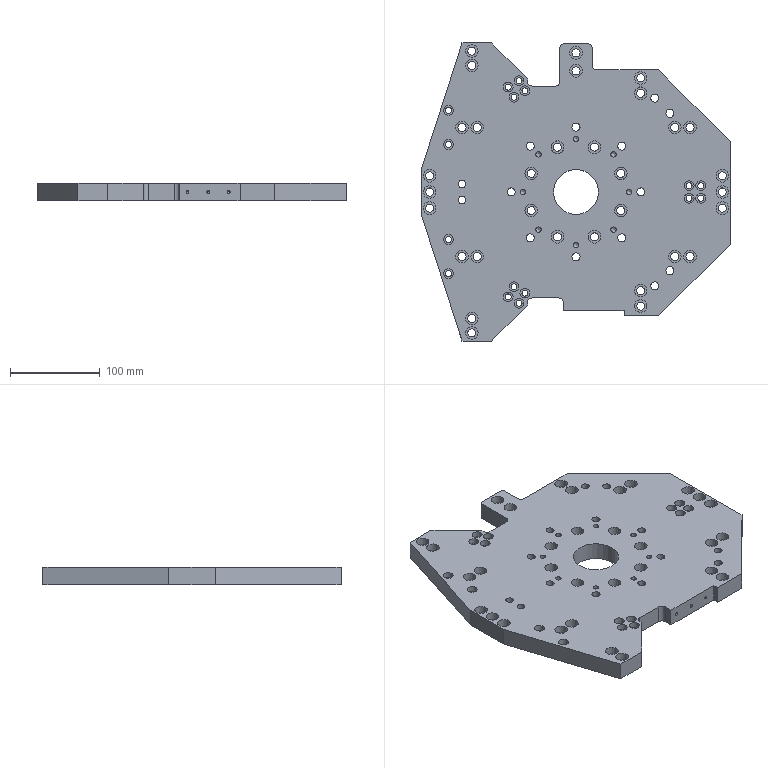Part | 1 solid | 236 faces | box 344 x 332 x 20 mm | volume 1561531 mm3 | cylinder 141 | plane 84 | cone 11 | commonest cylinder face diameters 9 x44 14 x44 6.6 x16 11 x16 6 x8 10 x7